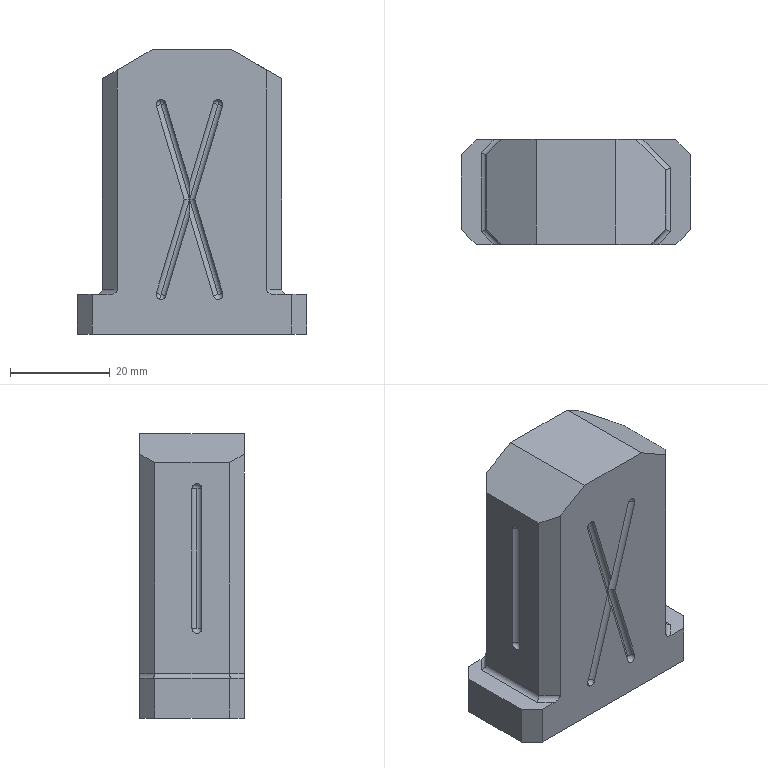Part | CATIA | 1 solid | 67 faces | box 46 x 21 x 57 mm | volume 41695 mm3 | cylinder 26 | sphere 21 | plane 20 | commonest cylinder face diameters 2 x26